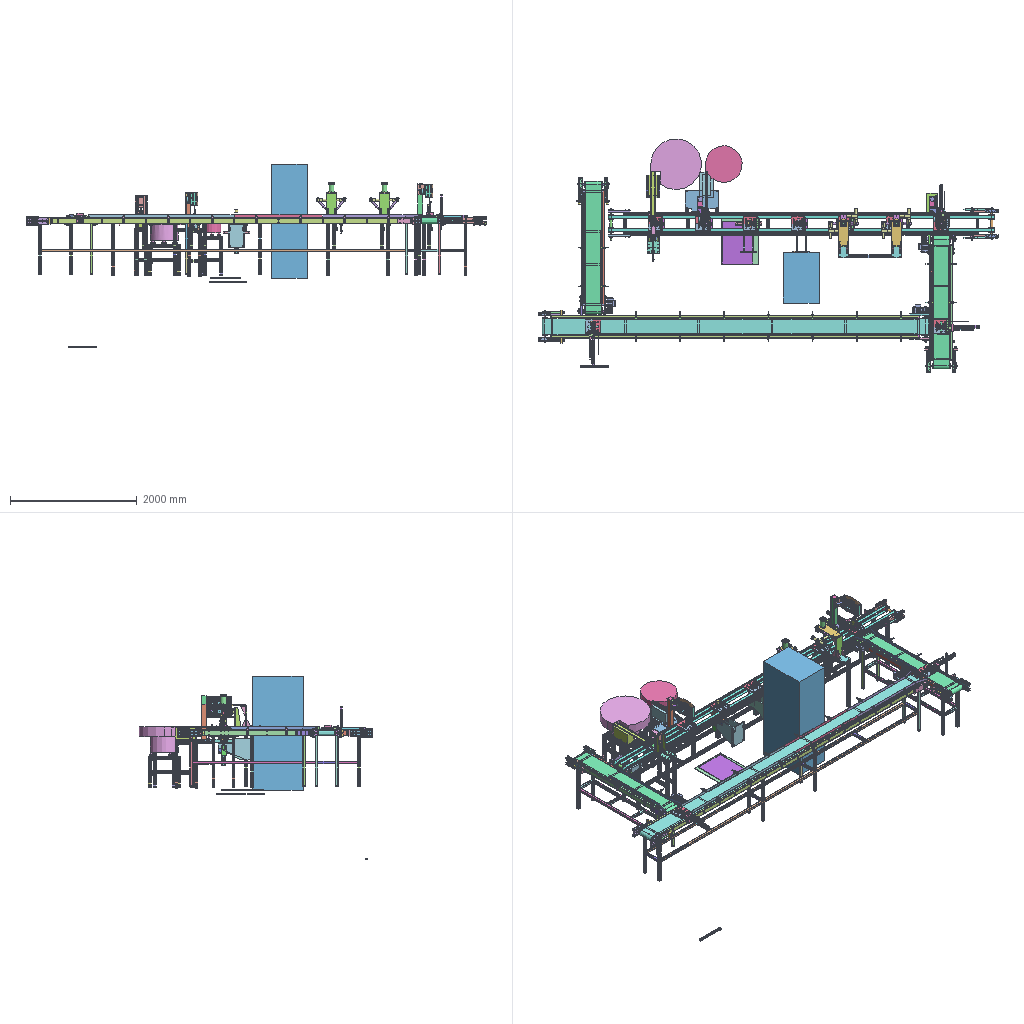Assembly | STEP file | 269 different items | 1938 placed | box 7251 x 3687 x 2899 mm
Parts list (item | name | quantity | parent item | size | volume):
1 | SN10_001_001_PLACA | x2 | in SN10_001_000_ESTEIRA | 400 x 25 x 100 mm | 770318 mm3
2 | SN10_001_002_SUPORTE | x4 | in SN10_001_000_ESTEIRA | 200 x 40 x 15 mm | 112660 mm3
3 | SN10_001_003_GUIA | x4 | in SN10_001_000_ESTEIRA | 200 x 11.9 x 27 mm | 60502 mm3
4 | SN10_001_004_PLACA | x2 | in SN10_001_000_ESTEIRA | 20 x 80 x 100 mm | 152757 mm3
5 | SN10_001_005_FUSO | x2 | in SN10_001_000_ESTEIRA | 402 x 20 x 20 mm | 117949 mm3
6 | SN10_001_006_EIXO | x1 | in SN10_001_000_ESTEIRA | 40 x 500.1 x 40 mm | 341783 mm3
7 | SN10_001_007_PLACA | x1 | in SN10_001_000_ESTEIRA | 345 x 25 x 90 mm | 704137 mm3
8 | SN10_001_008_EIXO | x1 | in SN10_001_000_ESTEIRA | 40 x 503.3 x 40 mm | 336623 mm3
9 | SN10_001_009_POLIA | x4 | in SN10_001_000_ESTEIRA | 92 x 80 x 92 mm | 413118 mm3
10 | SN10_001_010_PLACA | x1 | in SN10_001_000_ESTEIRA | 345 x 25 x 90 mm | 675174 mm3
11 | 1 | x2 | in SN10_001_011_ESTRUTURA | 5600 x 90 x 45 mm | 9330158 mm3
12 | 1_1 | x2 | in SN10_001_011_ESTRUTURA | 5510 x 45 x 45 mm | 4505764 mm3
13 | 1_2 | x4 | in SN10_001_011_ESTRUTURA | 855 x 45 x 45 mm | 699170 mm3
14 | 1_3 | x4 | in SN10_001_011_ESTRUTURA | 810 x 45 x 45 mm | 662372 mm3
15 | 1_4 | x2 | in SN10_001_011_ESTRUTURA | 680 x 45 x 45 mm | 556065 mm3
16 | 1_5 | x12 | in SN10_001_011_ESTRUTURA | 400 x 45 x 45 mm | 327097 mm3
17 | 1_6 | x4 | in SN10_001_011_ESTRUTURA | 300 x 45 x 45 mm | 245323 mm3
18 | 1_7 | x6 | in SN10_001_011_ESTRUTURA | 270 x 45 x 45 mm | 220791 mm3
19 | 1_8 | x4 | in SN10_001_011_ESTRUTURA | 245 x 45 x 45 mm | 200347 mm3
20 | 1_9 | x1 | in SN10_001_011_ESTRUTURA | 185 x 45 x 45 mm | 151282 mm3
21 | 1_10 | x1 | in SN10_001_011_ESTRUTURA | 520 x 45 x 45 mm | 425226 mm3
22 | 1_11 | x4 | in SN10_001_011_ESTRUTURA | 315 x 45 x 45 mm | 257589 mm3
23 | 1_12 | x1 | in SN10_001_011_ESTRUTURA | 985 x 45 x 45 mm | 805477 mm3
24 | 1_13 | x4 | in SN10_001_011_ESTRUTURA | 250 x 45 x 45 mm | 204436 mm3
25 | 1_14 | x2 | in SN10_001_011_ESTRUTURA | 855 x 45 x 45 mm | 699170 mm3
26 | 1_15 | x1 | in SN10_001_011_ESTRUTURA | 170 x 45 x 45 mm | 139016 mm3
27 | SN10_001_012_TRAVA | x1 | in SN10_001_000_ESTEIRA | 11 x 30 x 30 mm | 6549 mm3
28 | TU_20_TF_2_14a | x2 | in SN10_001_000_ESTEIRA | 35.3 x 92 x 97 mm | 122603 mm3
29 | 1_16 | x68 | in SN10_001_000_ESTEIRA, SN10_002_000_ESTEIRA, SN10_013_000_SISTEMA_ELEVATORIO | 13.4 x 13.4 x 2.5 mm | 205.865 mm3
30 | HABASIT_ESTEIRA | x2 | in SN10_001_000_ESTEIRA | 6090 x 50 x 90 mm | 1227646 mm3
31 | 1_17 | x36 | in SN10_001_000_ESTEIRA, SN10_002_000_ESTEIRA | 13 x 13 x 38 mm | 2414 mm3
32 | 1_18 | x48 | in SN10_001_000_ESTEIRA, SN10_002_000_ESTEIRA | 7.92 x 8 x 32 mm | 1366 mm3
33 | 1_19 | x40 | in SN10_001_000_ESTEIRA, SN10_002_000_ESTEIRA | 10 x 10 x 26 mm | 953.385 mm3
34 | 1_20 | x12 | in SN10_001_000_ESTEIRA, SN10_002_000_ESTEIRA | 13 x 13 x 43 mm | 2658 mm3
35 | 1_21 | x16 | in SN10_001_000_ESTEIRA | 19.4 x 8.5 x 45.7 mm | 2919 mm3
36 | 1_22 | x60 | in SN10_001_000_ESTEIRA, SN10_013_000_SISTEMA_ELEVATORIO, SN10_014_000_SISTEMA_BARRAGEM | 21 x 21 x 8 mm | 1207 mm3
37 | FYJ_3_4_TF_2_14a | x4 | in SN10_001_000_ESTEIRA, SN10_002_000_ESTEIRA, SN10_003_000_ESTEIRA | 33.3 x 86 x 86 mm | 78576 mm3
38 | 1_23 | x46 | in SN10_001_000_ESTEIRA, SN10_013_000_SISTEMA_ELEVATORIO, SN10_014_000_SISTEMA_BARRAGEM | 19.4 x 8.5 x 35.7 mm | 2417 mm3
39 | 1_24 | x4 | in SN10_001_000_ESTEIRA | 16.5 x 16.5 x 3 mm | 372.946 mm3
40 | 1_25 | x12 | in SN10_001_000_ESTEIRA, SN10_002_000_ESTEIRA | 16 x 16 x 50 mm | 4802 mm3
41 | 1_26 | x18 | in SN10_001_000_ESTEIRA, SN10_015_000_SISTEMA_TRANSFERENCIA, SN10_019_000_SISTEMA_DE_ABASTECIMENTO_ARRUELA | 10.4 x 10.4 x 2 mm | 101.14 mm3
42 | 1_27 | x4 | in SN10_001_000_ESTEIRA | 10 x 11.547 x 39 mm | 1326 mm3
43 | 1_28 | x1 | in SN10_001_000_ESTEIRA | 34.641 x 30 x 16 mm | 8431 mm3
44 | SN10_002_001_PLACA | x2 | in SN10_002_000_ESTEIRA | 315 x 25 x 90 mm | 605966 mm3
45 | SN10_002_002_PLACA | x2 | in SN10_002_000_ESTEIRA | 315 x 25 x 90 mm | 576590 mm3
46 | SN10_002_003_PLACA | x4 | in SN10_002_000_ESTEIRA | 20 x 80 x 100 mm | 152757 mm3
47 | SN10_002_004_PLACA | x4 | in SN10_002_000_ESTEIRA | 360 x 25 x 100 mm | 658656 mm3
48 | SN10_002_005_FUSO | x4 | in SN10_002_000_ESTEIRA | 270 x 35 x 35 mm | 89911 mm3
49 | SN10_002_006_GUIA | x8 | in SN10_002_000_ESTEIRA | 200 x 13.5 x 27 mm | 68797 mm3
50 | SN10_002_007_SUPORTE | x8 | in SN10_002_000_ESTEIRA | 200 x 40 x 15 mm | 112375 mm3
51 | SN10_002_008-01_TUBO_RETANGULAR | x2 | in SN10_002_008_ESTRUTURA | 1820 x 40 x 80 mm | 1167783 mm3
52 | SN10_002_008-02_TUBO_RETANGULAR | x4 | in SN10_002_008_ESTRUTURA | 360 x 40 x 80 mm | 211463 mm3
53 | SN10_002_008-03_TUBO_QUADRADO | x6 | in SN10_002_008_ESTRUTURA | 40 x 40 x 800 mm | 336658 mm3
54 | SN10_002_008-04_TUBO_QUADRADO | x4 | in SN10_002_008_ESTRUTURA | 1740 x 40 x 40 mm | 732232 mm3
55 | SN10_002_008-05_TUBO_QUADRADO | x8 | in SN10_002_008_ESTRUTURA | 40 x 280 x 40 mm | 117830 mm3
56 | SN10_002_008-06_TUBO_RETANGULAR | x4 | in SN10_002_008_ESTRUTURA | 40 x 280 x 80 mm | 185030 mm3
57 | SN10_002_008-07_PLACA | x8 | in SN10_002_008_ESTRUTURA | 34 x 34 x 19 mm | 18158 mm3
58 | SN10_002_008-09_TUBO_RETANGULAR | x2 | in SN10_002_008_ESTRUTURA | 1820 x 40 x 80 mm | 1165898 mm3
59 | SN10_002_008-10_TUBO_QUADRADO | x2 | in SN10_002_008_ESTRUTURA | 40 x 40 x 800 mm | 336658 mm3
60 | SN10_002_009-01_DISCO | x4 | in SN10_002_009_POLIA | 80 x 6.3 x 80 mm | 27788 mm3
61 | SN10_002_009-02_TUBO | x2 | in SN10_002_009_POLIA | 90 x 288.6 x 90 mm | 385332 mm3
62 | SN10_002_009-03_EIXO | x2 | in SN10_002_009_POLIA | 28 x 498.3 x 28 mm | 278975 mm3
63 | SN10_002_010-01_DISCO | x4 | in SN10_002_010_POLIA | 80 x 6.3 x 80 mm | 27788 mm3
64 | SN10_002_010-02_TUBO | x2 | in SN10_002_010_POLIA | 90 x 288.6 x 90 mm | 385332 mm3
65 | SN10_002_010-03_EIXO | x2 | in SN10_002_010_POLIA | 28 x 500.1 x 28 mm | 283207 mm3
66 | SN10_002_011_PLACA | x2 | in SN10_002_000_ESTEIRA | 40 x 10 x 60 mm | 22513 mm3
67 | 1_29 | x3 | in SN10_002_000_ESTEIRA, SN10_003_000_ESTEIRA | 256 x 153.5 x 121.5 mm | 2048036 mm3
68 | TU_20_TF_2_14a---(SKF) | x6 | in SN10_002_000_ESTEIRA, SN10_003_000_ESTEIRA | 35.3 x 92 x 97 mm | 122603 mm3
69 | ESTEIRA_002 | x2 | in SN10_002_000_ESTEIRA | 675.479 x 95 x 2102 mm | 2146084 mm3
70 | 1_30 | x194 | in SN10_002_000_ESTEIRA, SN10_015_000_SISTEMA_TRANSFERENCIA, SN10_016_000_SISTEMA_DE_GUIA, SN10_017_000_SISTEMA_DE_GUIA | 16.5 x 16.5 x 3 mm | 372.946 mm3
71 | 1_31 | x44 | in SN10_002_000_ESTEIRA, SN10_015_000_SISTEMA_TRANSFERENCIA | 16 x 16 x 90 mm | 7943 mm3
72 | 1_32 | x126 | in SN10_002_000_ESTEIRA, SN10_015_000_SISTEMA_TRANSFERENCIA, SN10_016_000_SISTEMA_DE_GUIA, SN10_017_000_SISTEMA_DE_GUIA | 19.63 x 17 x 8 mm | 1521 mm3
73 | SN10_003_001_PLACA | x1 | in SN10_003_000_ESTEIRA | 315 x 25 x 90 mm | 605966 mm3
74 | SN10_003_002_PLACA | x1 | in SN10_003_000_ESTEIRA | 315 x 25 x 90 mm | 578161 mm3
75 | SN10_003_003_PLACA | x2 | in SN10_003_000_ESTEIRA | 20 x 80 x 100 mm | 152757 mm3
76 | SN10_003_004_PLACA | x2 | in SN10_003_000_ESTEIRA | 360 x 25 x 100 mm | 661169 mm3
77 | SN10_003_005_FUSO | x2 | in SN10_003_000_ESTEIRA | 270 x 35 x 35 mm | 89911 mm3
78 | SN10_003_006_GUIA | x4 | in SN10_003_000_ESTEIRA | 200 x 13.5 x 27 mm | 68797 mm3
79 | SN10_003_007_SUPORTE | x4 | in SN10_003_000_ESTEIRA | 200 x 40 x 15 mm | 112375 mm3
80 | SN10_003_008-01_TUBO_RETANGULAR | x2 | in SN10_003_008_ESTRUTURA | 5820 x 40 x 80 mm | 3744159 mm3
81 | SN10_003_008-02_TUBO_RETANGULAR | x2 | in SN10_003_008_ESTRUTURA | 360 x 40 x 80 mm | 211463 mm3
82 | SN10_003_008-03_TUBO_QUADRADO | x4 | in SN10_003_008_ESTRUTURA | 40 x 40 x 800 mm | 336658 mm3
83 | SN10_003_008-04_TUBO_QUADRADO | x2 | in SN10_003_008_ESTRUTURA | 5740 x 40 x 40 mm | 2415524 mm3
84 | SN10_003_008-05_TUBO_QUADRADO | x6 | in SN10_003_008_ESTRUTURA | 40 x 280 x 40 mm | 117830 mm3
85 | SN10_003_008-06_TUBO_RETANGULAR | x4 | in SN10_003_008_ESTRUTURA | 40 x 280 x 80 mm | 185030 mm3
86 | SN10_003_008-07_PLACA | x8 | in SN10_003_008_ESTRUTURA | 34 x 34 x 19 mm | 18158 mm3
87 | SN10_003_008-08_TUBO_QUADRADO | x4 | in SN10_003_008_ESTRUTURA | 40 x 40 x 407 mm | 171275 mm3
88 | SN10_003_008-09_TUBO_QUADRADO | x4 | in SN10_003_008_ESTRUTURA | 40 x 40 x 353 mm | 148551 mm3
89 | SN10_003_009-01_DISCO | x2 | in SN10_003_009_POLIA | 80 x 6.3 x 80 mm | 27788 mm3
90 | SN10_003_009-02_TUBO | x1 | in SN10_003_009_POLIA | 90 x 288.6 x 90 mm | 385332 mm3
91 | SN10_003_009-03_EIXO | x1 | in SN10_003_009_POLIA | 28 x 498.3 x 28 mm | 277666 mm3
92 | SN10_003_010-01_DISCO | x2 | in SN10_003_010_POLIA | 80 x 6.3 x 80 mm | 27788 mm3
93 | SN10_003_010-02_TUBO | x1 | in SN10_003_010_POLIA | 90 x 288.6 x 90 mm | 385332 mm3
94 | SN10_003_010-03_EIXO | x1 | in SN10_003_010_POLIA | 28 x 500.1 x 28 mm | 283207 mm3
95 | ESTEIRA_003 | x1 | in SN10_003_000_ESTEIRA | 1498 x 95 x 6016 mm | 6146084 mm3
96 | BERCO_001 | x10 | in PRODUTO | 83.204 x 12 x 97.117 mm | 36018 mm3
97 | BERCO_002 | x10 | in PRODUTO | 247.817 x 12 x 265.596 mm | 428406 mm3
98 | BERCO_003 | x20 | in PRODUTO | 43.278 x 12 x 113.233 mm | 26889 mm3
99 | BERCO_004 | x10 | in PRODUTO | 223.963 x 12 x 154.905 mm | 182941 mm3
100 | BERCO_004_SIMETRICO | x10 | in PRODUTO | 226.019 x 12 x 152.848 mm | 182941 mm3
101 | BERCO_005 | x10 | in PRODUTO | 83.204 x 12 x 97.117 mm | 41261 mm3
102 | PARAFUSO M6x25 - DIN_912 | x40 | in PRODUTO | 31 x 10 x 10 mm | 1061 mm3
103 | PARAFUSO M4x20 - DIN_912 | x120 | in PRODUTO | 24 x 7 x 7 mm | 373.112 mm3
104 | 1_33 | x40 | in PRODUTO | 8.083 x 7 x 3.2 mm | 106.427 mm3
105 | PRODUTO_BUCHA | x10 | in Canoinha montada | 17 x 16 x 17 mm | 2259 mm3
106 | PRODUTO_PLACA | x10 | in Canoinha montada | - | -
107 | PRODUTO_ARRUELA | x13 | in Canoinha montada, SN10_006_000_ESTAGIO_2, SN10_019_000_SISTEMA_DE_ABASTECIMENTO_ARRUELA | 50 x 4.8 x 50 mm | 2970 mm3
108 | PRODUTO_PINO | x13 | in Canoinha montada, SN10_008_000_ESTAGIO_4 | 25 x 19 x 25 mm | 3402 mm3
109 | SN10_006_001_PILOTO | x1 | in SN10_006_000_ESTAGIO_2 | 30 x 100 x 30 mm | 30633 mm3
110 | SN10_006_002_PISADOR | x1 | in SN10_006_000_ESTAGIO_2 | 45.364 x 8 x 42.272 mm | 8699 mm3
111 | SN10_006_003_GUIA | x2 | in SN10_006_000_ESTAGIO_2 | 15.346 x 59 x 10.708 mm | 3098 mm3
112 | SN10_006_004_GAVETA | x1 | in SN10_006_000_ESTAGIO_2 | 122.344 x 12.5 x 315.126 mm | 195820 mm3
113 | SN10_006_005-01_PLACA | x1 | in SN10_006_005_CONJUNTO SOLDADO | 185 x 16 x 320 mm | 727969 mm3
114 | SN10_006_005-02_PLACA | x2 | in SN10_006_005_CONJUNTO SOLDADO | 50 x 91 x 15 mm | 63679 mm3
115 | SN10_006_005-03_REFORCO | x2 | in SN10_006_005_CONJUNTO SOLDADO | 16 x 80 x 310 mm | 276279 mm3
116 | SN10_006_006_SUPORTE | x2 | in SN10_006_000_ESTAGIO_2 | 65 x 158 x 19 mm | 192576 mm3
117 | SN10_006_007_PLACA | x1 | in SN10_006_000_ESTAGIO_2 | 185 x 290 x 25.5 mm | 1268482 mm3
118 | 19211 DSNU-20-80-P-A | x1 | in SN10_006_000_ESTAGIO_2 | 36.95 x 32 x 292 mm | 57538 mm3
119 | 19210 DSNU-20-50-P-A-----(asm_0_1) | x1 | in SN10_006_000_ESTAGIO_2 | 36.95 x 32 x 232 mm | 60932 mm3
120 | SHS15C-1SS-155 | x1 | in SN10_006_000_ESTAGIO_2 | 155 x 47 x 24.001 mm | 62079 mm3
121 | 2062 FK-M8 | x1 | in SN10_006_000_ESTAGIO_2 | 17 x 19 x 49 mm | 7068 mm3
122 | 1_34 | x3 | in SN10_006_000_ESTAGIO_2 | 25 x 45 x 54 mm | 12239 mm3
123 | PROJECTION BASE 1 WASHER | x2 | in MACHINE BASE PROJECTION 1 WASHER | 205 x 160 x 169 mm | 2313406 mm3
124 | SN10_013_001_PLACA | x6 | in SN10_013_000_SISTEMA_ELEVATORIO | 19 x 170 x 140 mm | 426435 mm3
125 | SN10_013_002_PINO | x12 | in SN10_013_000_SISTEMA_ELEVATORIO | 43 x 15 x 15 mm | 6907 mm3
126 | SN10_013_003_PINO_CONICO | x12 | in SN10_013_000_SISTEMA_ELEVATORIO | 58 x 15 x 15 mm | 7980 mm3
127 | MACHINE BASE PROJECTION 1 | x1 | in MACHINE BASE PROJECTION 1 WASHER | 260 x 360 x 535 mm | 5517318 mm3
128 | UPPER ELECTRODE PROJECTION 1 | x1 | in MACHINE BASE PROJECTION 1 WASHER | 48 x 48 x 50 mm | 90478 mm3
129 | base da maquina | x1 | in MACHINE BASE PROJECTION 1 WASHER | 486.837 x 663.677 x 10 mm | 3231029 mm3
130 | floor | x1 | in MACHINE BASE PROJECTION 1 WASHER | 586.14 x 746.049 x 10 mm | 4372895 mm3
131 | COMPOUND | x1 | in MACHINE BASE PROJECTION 1 WASHER | - | -
132 | SOLID | x1 | in SN10_007_001-01_PLACA | 209.056 x 12 x 193.596 mm | 339030 mm3
133 | COMPOUND | x1 | in SN10_007_001-01_PLACA | - | -
134 | SN10_007_001-02_PLACA | x2 | in Projection lift assembly | 44.646 x 150 x 159.048 mm | 285095 mm3
135 | SN10_007_001-03_PLACA | x1 | in Projection lift assembly | 103.364 x 12 x 171.387 mm | 133438 mm3
136 | SN10_007_005_PLACA | x1 | in Projection lift assembly | 168.139 x 12 x 110.165 mm | 127729 mm3
137 | 163371 DNC-50-50-PPV-A | x2 | in Projection lift assembly, SN10_009_000_ESTAGIO_5 | 64 x 64 x 279 mm | 523185 mm3
138 | placa de celeron | x1 | in Projection lift assembly | 12 x 180 x 160 mm | 345600 mm3
139 | SUPORTE | x2 | in Projection lift assembly | 165 x 80 x 12 mm | 153227 mm3
140 | SHIM SUPPORT | x2 | in Projection lift assembly | 130 x 32.9 x 50 mm | 166423 mm3
141 | COMPOUND | x1 | - | - | -
142 | SN10_008_001_PLACA | x1 | in SN10_008_000_ESTAGIO_4 | 520 x 340 x 15 mm | 2444343 mm3
143 | SN10_008_002_SUPORTE | x1 | in SN10_008_000_ESTAGIO_4 | 38 x 65 x 110 mm | 83544 mm3
144 | SN10_008_003_SUPORTE | x1 | in SN10_008_000_ESTAGIO_4 | 20 x 90 x 165.5 mm | 85051 mm3
145 | SN10_008_004_SUPORTE | x1 | in SN10_008_000_ESTAGIO_4 | 33 x 30 x 90 mm | 36222 mm3
146 | SN10_008_006-01_TUBO_QUADRADO | x1 | in SN10_008_006_CONJUNTO_SOLDADO | 80 x 80 x 546 mm | 491849 mm3
147 | SN10_008_006-02_PLACA | x2 | in SN10_008_006_CONJUNTO_SOLDADO, Copy (1) of SN10_008_006_CONJUNTO_SOLDADO | 80 x 240 x 15 mm | 283759 mm3
148 | SN10_008_006-03_PLACA | x2 | in SN10_008_006_CONJUNTO_SOLDADO, Copy (1) of SN10_008_006_CONJUNTO_SOLDADO | 80 x 15 x 160 mm | 188410 mm3
149 | SN10_008_006-04_TAMPA | x2 | in SN10_008_006_CONJUNTO_SOLDADO, Copy (1) of SN10_008_006_CONJUNTO_SOLDADO | 80 x 80 x 3 mm | 19107 mm3
150 | SN10_008_007-01_PLACA | x2 | in SN10_008_007_CONJUNTO_SOLDADO, Copy (1) of SN10_008_007_CONJUNTO_SOLDADO | 15 x 80 x 160 mm | 188607 mm3
151 | SN10_008_007-02_PLACA | x1 | in SN10_008_007_CONJUNTO_SOLDADO | 75 x 15 x 160 mm | 174675 mm3
152 | SN10_008_007-03_REFORCO | x1 | in SN10_008_007_CONJUNTO_SOLDADO | 65 x 80 x 16 mm | 55325 mm3
153 | 189171_ESG_10_SN_HA_QS_2_14b | x1 | in SN10_008_000_ESTAGIO_4 | 14 x 34.4 x 16.166 mm | 3340 mm3
154 | - | x12 | in P533616_HSP_25_AP_SD | 8.5 x 25 x 8.5 mm | 625.305 mm3
155 | - | x4 | in P533616_HSP_25_AP_SD | 82.749 x 20 x 200 mm | 243031 mm3
156 | - | x2 | in P533616_HSP_25_AP_SD | 360 x 200 x 36.871 mm | 145158 mm3
157 | - | x12 | in P533616_HSP_25_AP_SD | 8.5 x 17 x 8.5 mm | 468.225 mm3
158 | - | x2 | in P533616_HSP_25_AP_SD | 50 x 60 x 12.5 mm | 28207 mm3
159 | - | x4 | in P533616_HSP_25_AP_SD | 75.3 x 12 x 12 mm | 6099 mm3
160 | - | x4 | in P533616_HSP_25_AP_SD | 15 x 17.321 x 25 mm | 2729 mm3
161 | Senkschraube_DIN_965_M3x4 | x4 | in P533616_HSP_25_AP_SD | 5.6 x 4 x 5.6 mm | 33.649 mm3
162 | - | x4 | in P533616_HSP_25_AP_SD | 9 x 6.5 x 50 mm | 1500 mm3
163 | - | x2 | in P533616_HSP_25_AP_SD | 24 x 47 x 45 mm | 16099 mm3
164 | - | x4 | in P533616_HSP_25_AP_SD | 13 x 13 x 26.5 mm | 1380 mm3
165 | - | x22 | in P533616_HSP_25_AP_SD | 8.5 x 21 x 8.5 mm | 546.765 mm3
166 | - | x2 | in P533616_HSP_25_AP_SD | 18 x 143 x 110 mm | 148333 mm3
167 | - | x2 | in P533616_HSP_25_AP_SD | 24 x 47 x 45 mm | 16099 mm3
168 | - | x2 | in P533616_HSP_25_AP_SD | 110 x 143 x 18 mm | 148402 mm3
169 | - | x2 | in P533616_HSP_25_AP_SD | 19 x 19 x 50 mm | 7855 mm3
170 | - | x22 | in P533616_HSP_25_AP_SD | 7 x 14 x 7 mm | 255.725 mm3
171 | - | x4 | in P533616_HSP_25_AP_SD | 26.5 x 13 x 13 mm | 1379 mm3
172 | - | x6 | in P533616_HSP_25_AP_SD | 13 x 4 x 15.011 mm | 436.424 mm3
173 | Scheibe_DIN_125_1_B_8_4 | x2 | in P533616_HSP_25_AP_SD | 16 x 1.6 x 16 mm | 224.209 mm3
174 | - | x2 | in P533616_HSP_25_AP_SD | 93 x 54 x 12 mm | 19290 mm3
175 | - | x2 | in P533616_HSP_25_AP_SD | 49 x 24 x 49 mm | 37752 mm3
176 | - | x2 | in P533616_HSP_25_AP_SD | 23.2 x 10 x 250 mm | 48053 mm3
177 | - | x2 | in P533616_HSP_25_AP_SD | 15.5 x 26 x 250 mm | 83813 mm3
178 | - | x2 | in P533616_HSP_25_AP_SD | 30 x 123.5 x 10 mm | 18320 mm3
179 | - | x2 | in P533616_HSP_25_AP_SD | 28 x 28 x 35.5 mm | 17370 mm3
180 | - | x8 | in P533616_HSP_25_AP_SD | 8.5 x 30 x 8.5 mm | 723.48 mm3
181 | - | x2 | in P533616_HSP_25_AP_SD | 105.5 x 83.2 x 83.2 mm | 387227 mm3
182 | - | x2 | in P533616_HSP_25_AP_SD | 20 x 200 x 340 mm | 654587 mm3
183 | - | x2 | in P533616_HSP_25_AP_SD | 250 x 10 x 23.2 mm | 48160 mm3
184 | 5_ESTAGIO_001 | x1 | in SN10_009_000_ESTAGIO_5 | 82.899 x 120 x 82.899 mm | 294480 mm3
185 | 5_ESTAGIO_002 | x1 | in SN10_009_000_ESTAGIO_5 | 20 x 40 x 20 mm | 12566 mm3
186 | 5_ESTAGIO_003-01 | x1 | in 5_ESTAGIO_003 | 209.056 x 20 x 193.596 mm | 576000 mm3
187 | 5_ESTAGIO_003-02 | x2 | in 5_ESTAGIO_003 | 48.561 x 150 x 159.871 mm | 384000 mm3
188 | 5_ESTAGIO_003-03 | x1 | in 5_ESTAGIO_003 | 119.022 x 16 x 174.677 mm | 225280 mm3
189 | 5_ESTAGIO_004-01 | x2 | in 5_ESTAGIO_004 | 125.479 x 285 x 508.106 mm | 2421288 mm3
190 | 5_ESTAGIO_004-02 | x1 | in 5_ESTAGIO_004 | 263.449 x 360 x 74.068 mm | 1908000 mm3
191 | 5_ESTAGIO_005 | x1 | in SN10_009_000_ESTAGIO_5 | 173.032 x 16 x 111.193 mm | 184694 mm3
192 | SHS15C12030_Track | x4 | in SHS15C1SS120300PB1021B27.8000 | 120 x 13 x 15 mm | 19221 mm3
193 | SHS15CSSPB1021B_Slide25_55 | x4 | in SHS15C1SS120300PB1021B27.8000 | 64.4 x 21 x 47 mm | 41845 mm3
194 | 5_ESTAGIO_MAQUINA | x1 | in SN10_009_000_ESTAGIO_5 | 717.439 x 1800 x 899.09 mm | 813600000 mm3
195 | SN10_010_001_SUPORTE | x8 | in SN10_010_000_ESTAGIO_6, SN10_011_000_ESTAGIO_7 | 40 x 260 x 50 mm | 323681 mm3
196 | SN10_010_002_SUPORTE | x2 | in SN10_010_000_ESTAGIO_6, SN10_011_000_ESTAGIO_7 | 100 x 300 x 19 mm | 495492 mm3
197 | SN10_010_003_SUPORTE | x4 | in SN10_010_000_ESTAGIO_6, SN10_011_000_ESTAGIO_7 | 40 x 50 x 75 mm | 100062 mm3
198 | SN10_010_004_EIXO | x2 | in SN10_010_000_ESTAGIO_6, SN10_011_000_ESTAGIO_7 | 60 x 60 x 50 mm | 51834 mm3
199 | SN10_010_005-01_PLACA | x2 | in SN10_010_005_CONJUNTO_SOLDADO | 150 x 80 x 19 mm | 223453 mm3
200 | SN10_010_005-02_PLACA | x2 | in SN10_010_005_CONJUNTO_SOLDADO | 150 x 19 x 362.5 mm | 1033125 mm3
201 | SN10_010_005-03_REFORCO | x12 | in SN10_010_005_CONJUNTO_SOLDADO | 19 x 70 x 137 mm | 117421 mm3
202 | SN10_010_005-04_PLACA | x2 | in SN10_010_005_CONJUNTO_SOLDADO | 150 x 360 x 20 mm | 1065035 mm3
203 | SN10_010_006_PLACA | x2 | in SN10_010_000_ESTAGIO_6, SN10_011_000_ESTAGIO_7 | 150 x 425 x 19 mm | 1079785 mm3
204 | TOCHA_DE_SOLDA_TBI | x4 | in SN10_010_000_ESTAGIO_6, SN10_011_000_ESTAGIO_7 | 38 x 348 x 38 mm | 253151 mm3
205 | COMPOUND | x2 | in PE0902 | - | -
206 | SOLID | x2 | in PE0902 | 192.5 x 90 x 90 mm | 903685 mm3
207 | COMPOUND | x2 | in P0405300101 | - | -
208 | SOLID | x2 | in P0405300101 | 92 x 92 x 23.5 mm | 95291 mm3
209 | PARAFUSO_DIN 912_M8x30 | x2 | in SN10_010_000_ESTAGIO_6, SN10_011_000_ESTAGIO_7 | 38 x 13 x 13 mm | 2340 mm3
210 | 1254052_DHPS_35_A_2_14a---(CORPO) | x1 | in 1254052_DHPS_35_A_2_14a---(FESTO) | 45 x 110 x 88 mm | 385096 mm3
211 | 1254052_DHPS_35_A_2_14a---(GARRA) | x2 | in 1254052_DHPS_35_A_2_14a---(FESTO) | 20 x 55.5 x 42.5 mm | 31534 mm3
212 | SN10_012_001_GARRA | x2 | in SN10_012_000_ESTAGIO_8 | 19 x 39 x 63 mm | 23093 mm3
213 | 540883_HAPG_72_B_2_14b | x1 | in SN10_012_000_ESTAGIO_8 | 47 x 60 x 63.5 mm | 42972 mm3
214 | SN10_012_002_ADAPTADOR | x1 | in SN10_012_000_ESTAGIO_8 | 50 x 90 x 15 mm | 62180 mm3
215 | ISO 4762 SCREW M8x20 STEEL HEXAGON SOCKET HEAD CAP | x2 | in SN10_012_000_ESTAGIO_8 | 28 x 13 x 13 mm | 1862 mm3
216 | Copy (1) of SN10_008_006-01_TUBO_QUADRADO | x1 | in Copy (1) of SN10_008_006_CONJUNTO_SOLDADO | 80 x 80 x 507.179 mm | 456879 mm3
217 | Copy (1) of SN10_008_007-02_PLACA | x1 | in Copy (1) of SN10_008_007_CONJUNTO_SOLDADO | 120 x 15 x 160 mm | 282675 mm3
218 | Copy (1) of SN10_008_007-03_REFORCO | x1 | in Copy (1) of SN10_008_007_CONJUNTO_SOLDADO | 110 x 80 x 16 mm | 89525 mm3
219 | SN10_012_002_PLACA | x1 | in SN10_012_000_ESTAGIO_8 | 170 x 295 x 15 mm | 749791 mm3
220 | 189654 HMBN-5-M5-189654 HMBN-5-M5 | x2 | in SN10_012_000_ESTAGIO_8 | 7.6 x 5.445 x 12 mm | 233.461 mm3
221 | SN10_013_004_PLACA | x5 | in SN10_013_000_SISTEMA_ELEVATORIO | 10 x 360 x 100 mm | 258052 mm3
222 | - | x5 | in 170858 DFM-32-50-P-A-GF---(FESTO) | 98 x 49 x 110 mm | 384442 mm3
223 | - | x5 | in 170858 DFM-32-50-P-A-GF---(FESTO) | 131 x 47 x 108 mm | 163478 mm3
224 | 1_35 | x20 | in SN10_013_000_SISTEMA_ELEVATORIO | 8.5 x 8.5 x 35 mm | 827.103 mm3
225 | 1_36 | x20 | in SN10_013_000_SISTEMA_ELEVATORIO | 13 x 13 x 33 mm | 2162 mm3
226 | 1_37 | x24 | in SN10_013_000_SISTEMA_ELEVATORIO, SN10_019_000_SISTEMA_DE_ABASTECIMENTO_ARRUELA | 8.3 x 8.3 x 1.5 mm | 44.494 mm3
227 | SN10_014_001_PINO | x6 | in SN10_014_000_SISTEMA_BARRAGEM | 20 x 20 x 40 mm | 11102 mm3
228 | SN10_014_002-01_PLACA | x6 | in SN10_014_002_CONJUNTO_SOLDADO | 50 x 360 x 12.5 mm | 206301 mm3
229 | SN10_014_002-02_TUBO | x6 | in SN10_014_002_CONJUNTO_SOLDADO | 50 x 50 x 80 mm | 129371 mm3
230 | - | x6 | in 19210 DSNU-20-50-P-A-----(FESTO) | 27 x 27 x 158 mm | 40169 mm3
231 | - | x6 | in 19210 DSNU-20-50-P-A-----(FESTO) | 20 x 20 x 142 mm | 8430 mm3
232 | SN10_015_001_CHAPA_DOBRADA | x3 | in SN10_015_000_SISTEMA_TRANSFERENCIA | 485 x 210 x 19 mm | 177968 mm3
233 | SN10_015_002_PLACA | x3 | in SN10_015_000_SISTEMA_TRANSFERENCIA | 25 x 110 x 160 mm | 292195 mm3
234 | SN10_015_003_GUIA | x3 | in SN10_015_000_SISTEMA_TRANSFERENCIA | 380 x 10 x 10 mm | 29333 mm3
235 | SN10_015_004_BUCHA | x3 | in SN10_015_000_SISTEMA_TRANSFERENCIA | 25 x 20 x 20 mm | 5796 mm3
236 | 163314 DNC-32-320-PPV-A---(FESTO)_CORPO | x3 | in 163314 DNC-32-320-PPV-A---(FESTO) | 45 x 45 x 436 mm | 470774 mm3
237 | 163314 DNC-32-320-PPV-A---(FESTO)_HASTE | x3 | in 163314 DNC-32-320-PPV-A---(FESTO) | 32 x 32 x 415 mm | 50245 mm3
238 | 1_38 | x12 | in SN10_015_000_SISTEMA_TRANSFERENCIA | 10 x 10 x 46 mm | 1516 mm3
239 | SN10_016_001-01_CHAPA | x4 | in SN10_016_001_GUIA | 56.488 x 1320 x 45 mm | 179098 mm3
240 | SN10_016_001-02_BLOCO | x8 | in SN10_016_001_GUIA | 20 x 20 x 45 mm | 16964 mm3
241 | SN10_016_002_SUPORTE | x22 | in SN10_016_000_SISTEMA_DE_GUIA, SN10_017_000_SISTEMA_DE_GUIA | 3 x 30 x 135 mm | 11295 mm3
242 | SN10_016_003_EIXO | x22 | in SN10_016_000_SISTEMA_DE_GUIA, SN10_017_000_SISTEMA_DE_GUIA | 120 x 10 x 10 mm | 9417 mm3
243 | 1_39 | x16 | in SN10_016_000_SISTEMA_DE_GUIA | 16 x 16 x 80 mm | 7147 mm3
244 | SN10_017_001-01_CHAPA | x2 | in SN10_017_001_GUIA | 1494 x 56.488 x 45 mm | 202588 mm3
245 | SN10_017_001-02_BLOCO | x14 | in SN10_017_001_GUIA, SN10_017_002_GUIA, SN10_017_003_GUIA | 20 x 20 x 45 mm | 17008 mm3
246 | SN10_017_002-01_CHAPA | x2 | in SN10_017_002_GUIA | 1382 x 3 x 45 mm | 186570 mm3
247 | SN10_017_003-01_CHAPA | x2 | in SN10_017_003_GUIA | 2283 x 3 x 45 mm | 308205 mm3
248 | bosch_3842990520_4ea8orsd7ktxgd8l9ys4v93ta | x4 | in SN10_019_001_ALUMINUM_STRUCTURE | 485 x 45 x 45 mm | 396605 mm3
249 | bosch_3842990520_4g1k76bwvav0hbf1r78r1itfr | x11 | in SN10_019_001_ALUMINUM_STRUCTURE | 410 x 45 x 45 mm | 335275 mm3
250 | bosch_3842529383_ce331vk4hpgd1h6tci1llkgc1 | x20 | in SN10_019_001_ALUMINUM_STRUCTURE | 38 x 47.7 x 47.7 mm | 18640 mm3
251 | bosch_3842990520_1jcimurca0n3y5im9bxpmvpzt | x8 | in SN10_019_002_ALUMINUM_STRUCTURE, SN10_020_002_ALUMINUM_STRUCTURE | 740 x 45 x 45 mm | 605130 mm3
252 | bosch_3842990520_2f8lx2d0pfreq4lhyqg120tj6 | x12 | in SN10_019_002_ALUMINUM_STRUCTURE, SN10_020_002_ALUMINUM_STRUCTURE | 270 x 45 x 45 mm | 220791 mm3
253 | bosch_3842990520_bbw6j7b49i4caf90m9u0fayle | x8 | in SN10_019_002_ALUMINUM_STRUCTURE, SN10_020_002_ALUMINUM_STRUCTURE | 122 x 45 x 45 mm | 99765 mm3
254 | SN10_019_003_SUPORTE | x1 | in SN10_019_000_SISTEMA_DE_ABASTECIMENTO_ARRUELA | 16 x 161 x 147.15 mm | 54772 mm3
255 | 2_ESTAGIO_006-01 | x1 | in 2_ESTAGIO_006 | 85.161 x 5 x 93.664 mm | 26952 mm3
256 | 2_ESTAGIO_006-02 | x1 | in 2_ESTAGIO_006 | 25.4 x 30 x 25.4 mm | 10290 mm3
257 | 2_ESTAGIO_010 | x1 | in SN10_019_000_SISTEMA_DE_ABASTECIMENTO_ARRUELA | 109.627 x 12.7 x 98.805 mm | 71258 mm3
258 | 2_ESTAGIO_005 | x1 | in SN10_019_000_SISTEMA_DE_ABASTECIMENTO_ARRUELA | 10 x 15 x 10 mm | 994.545 mm3
259 | 19183 DSNU-10-10-P-A | x1 | in SN10_019_000_SISTEMA_DE_ABASTECIMENTO_ARRUELA | 15 x 15 x 106 mm | 9040 mm3
260 | CALHA_VIBRATORIA_ARRUELA | x1 | in SN10_019_000_SISTEMA_DE_ABASTECIMENTO_ARRUELA | 700 x 132 x 200 mm | 8382102 mm3
261 | ALIMENTADOR_ARRUELA | x1 | in SN10_019_000_SISTEMA_DE_ABASTECIMENTO_ARRUELA | 800 x 800 x 450 mm | 113086598 mm3
262 | DIN_912 - M5x16 | x4 | in SN10_019_000_SISTEMA_DE_ABASTECIMENTO_ARRUELA | 21 x 8.5 x 8.5 mm | 538.828 mm3
263 | DISCO_BASE_ALIMENTADOR_ARRUELA | x3 | in SN10_019_000_SISTEMA_DE_ABASTECIMENTO_ARRUELA | 70 x 70 x 10 mm | 27729 mm3
264 | bosch_3842990520_3kqsoefwhpgbs6igd9j6s2bp3 | x4 | in SN10_020_001_ALUMINUM_STRUCTURE | 610 x 45 x 45 mm | 498823 mm3
265 | bosch_3842990520_akhtc56kol25hyvavz80csddc | x11 | in SN10_020_001_ALUMINUM_STRUCTURE | 255 x 45 x 45 mm | 208524 mm3
266 | ALIMENTADOR_PINO | x1 | in SN10_020_000_SISTEMA_DE_ABASTECIMENTO_PINO | 580 x 580 x 320 mm | 38023743 mm3
267 | CALHA_VIBRATORIA_PINO | x1 | in SN10_020_000_SISTEMA_DE_ABASTECIMENTO_PINO | 600 x 212 x 235 mm | 9636960 mm3
268 | DISCO_BASE_ALIMENTADOR_PINO | x3 | in SN10_020_000_SISTEMA_DE_ABASTECIMENTO_PINO | 52 x 52 x 10 mm | 17173 mm3
269 | PERFIL_30X30_450 | x2 | in _SN10_000_000_PROJETO_CANOINHA_KEIPER | 450 x 30 x 30 mm | 139687 mm3
Placements (level | parent | child | x y z in mm | rotation matrix by rows), first 188 of 2061 lines:
1 | Canoinha | _SN10_000_000_PROJETO_CANOINHA_KEIPER | 0.0 0.0 0.0 | 1 0 0 0 1 0 0 0 1
2 | _SN10_000_000_PROJETO_CANOINHA_KEIPER | SN10_001_000_ESTEIRA | 0.0 0.0 0.0 | 1 0 0 0 1 0 0 0 1
3 | SN10_001_000_ESTEIRA | SN10_001_001_PLACA | 6000.0 -0.0 0.0 | -1 0 0 0 -1 0 0 0 1
3 | SN10_001_000_ESTEIRA | SN10_001_001_PLACA | 6000.0 -0.0 0.0 | -1 0 0 0 1 0 0 0 -1
3 | SN10_001_000_ESTEIRA | SN10_001_002_SUPORTE | 6000.0 -0.0 0.0 | -1 0 0 0 -1 0 0 0 1
3 | SN10_001_000_ESTEIRA | SN10_001_002_SUPORTE | 6000.0 -0.0 0.0 | 1 0 0 0 -1 0 0 0 -1
3 | SN10_001_000_ESTEIRA | SN10_001_002_SUPORTE | 6000.0 -0.0 0.0 | 1 0 0 0 1 0 0 0 1
3 | SN10_001_000_ESTEIRA | SN10_001_002_SUPORTE | 6000.0 -0.0 0.0 | -1 0 0 0 1 0 0 0 -1
3 | SN10_001_000_ESTEIRA | SN10_001_003_GUIA | 6000.0 -0.0 0.0 | -1 0 0 0 -1 0 0 0 1
3 | SN10_001_000_ESTEIRA | SN10_001_003_GUIA | 6000.0 -0.0 0.0 | 1 0 0 0 -1 0 0 0 -1
3 | SN10_001_000_ESTEIRA | SN10_001_003_GUIA | 6000.0 -0.0 0.0 | 1 0 0 0 1 0 0 0 1
3 | SN10_001_000_ESTEIRA | SN10_001_003_GUIA | 6000.0 -0.0 0.0 | -1 0 0 0 1 0 0 0 -1
3 | SN10_001_000_ESTEIRA | SN10_001_004_PLACA | 6000.0 -0.0 0.0 | -1 0 0 0 -1 0 0 0 1
3 | SN10_001_000_ESTEIRA | SN10_001_004_PLACA | 6000.0 -0.0 0.0 | -1 0 0 0 1 0 0 0 -1
3 | SN10_001_000_ESTEIRA | SN10_001_005_FUSO | 6000.0 -0.0 0.0 | -1 0 0 0 -1 0 0 0 1
3 | SN10_001_000_ESTEIRA | SN10_001_005_FUSO | 6000.0 442.7 0.0 | -1 0 0 0 -1 0 0 0 1
3 | SN10_001_000_ESTEIRA | SN10_001_006_EIXO | 6000.0 -0.0 0.0 | -1 0 0 0 -1 0 0 0 1
3 | SN10_001_000_ESTEIRA | SN10_001_007_PLACA | 6000.0 -0.0 0.0 | -1 0 0 0 1 0 0 0 -1
3 | SN10_001_000_ESTEIRA | SN10_001_008_EIXO | 6000.0 -0.0 0.0 | -1 0 0 0 -1 0 0 0 1
3 | SN10_001_000_ESTEIRA | SN10_001_009_POLIA | 6000.0 -0.0 0.0 | -1 0 0 0 -1 0 0 0 1
3 | SN10_001_000_ESTEIRA | SN10_001_009_POLIA | 6000.0 -200.0 0.0 | -1 0 0 0 -1 0 0 0 1
3 | SN10_001_000_ESTEIRA | SN10_001_009_POLIA | 12000.0 -0.0 0.0 | -1 0 0 0 -1 0 0 0 1
3 | SN10_001_000_ESTEIRA | SN10_001_009_POLIA | 12000.0 -200.0 0.0 | -1 0 0 0 -1 0 0 0 1
3 | SN10_001_000_ESTEIRA | SN10_001_010_PLACA | 6000.0 -0.0 0.0 | -1 0 0 0 -1 0 0 0 1
3 | SN10_001_000_ESTEIRA | SN10_001_011_ESTRUTURA | 0.0 0.0 0.0 | 1 0 0 0 1 0 0 0 1
4 | SN10_001_011_ESTRUTURA | 1 | 200.0 157.5 0.0 | 1 0 0 0 0 1 0 -1 0
4 | SN10_001_011_ESTRUTURA | 1 | 200.0 -157.5 0.0 | 1 0 0 0 0 1 0 -1 0
4 | SN10_001_011_ESTRUTURA | 1_1 | 134.371 157.5 -467.5 | 1 0 0 0 1 0 0 0 1
4 | SN10_001_011_ESTRUTURA | 1_1 | 134.371 -157.5 -467.5 | 1 0 0 0 1 0 0 0 1
4 | SN10_001_011_ESTRUTURA | 1_2 | 4552.5 -517.5 0.0 | 0 0 -1 0 -1 0 -1 0 0
4 | SN10_001_011_ESTRUTURA | 1_2 | 736.371 -447.5 -0.0 | 0 0 -1 0 -1 0 -1 0 0
4 | SN10_001_011_ESTRUTURA | 1_3 | 222.5 157.5 -855.0 | 0 0 1 0 -1 0 1 0 0
4 | SN10_001_011_ESTRUTURA | 1_3 | 222.5 -157.5 -855.0 | 0 0 1 0 -1 0 1 0 0
4 | SN10_001_011_ESTRUTURA | 1_3 | 5777.5 157.5 -855.0 | 0 0 1 0 -1 0 1 0 0
4 | SN10_001_011_ESTRUTURA | 1_3 | 5777.5 -157.5 -855.0 | 0 0 1 0 -1 0 1 0 0
4 | SN10_001_011_ESTRUTURA | 1_4 | 1195.588 502.5 -175 | 0 0 1 0 1 0 -1 0 0
4 | SN10_001_011_ESTRUTURA | 1_4 | 1670.588 502.5 -175 | 0 0 1 0 1 0 -1 0 0
4 | SN10_001_011_ESTRUTURA | 1_5 | 707.0 157.5 -445.0 | 0 0 1 0 -1 0 1 0 0
4 | SN10_001_011_ESTRUTURA | 1_5 | 1195.588 157.5 -445.0 | 0 0 1 0 -1 0 1 0 0
4 | SN10_001_011_ESTRUTURA | 1_5 | 3707.0 157.5 -445.0 | 0 0 1 0 -1 0 1 0 0
4 | SN10_001_011_ESTRUTURA | 1_5 | 4457.0 157.5 -445.0 | 0 0 1 0 -1 0 1 0 0
4 | SN10_001_011_ESTRUTURA | 1_5 | 707.0 -157.5 -445.0 | 0 0 1 0 -1 0 1 0 0
4 | SN10_001_011_ESTRUTURA | 1_5 | 1457.0 -157.5 -445.0 | 0 0 1 0 -1 0 1 0 0
4 | SN10_001_011_ESTRUTURA | 1_5 | 3707.0 -157.5 -445.0 | 0 0 1 0 -1 0 1 0 0
4 | SN10_001_011_ESTRUTURA | 1_5 | 4457.0 -157.5 -445.0 | 0 0 1 0 -1 0 1 0 0
4 | SN10_001_011_ESTRUTURA | 1_6 | 1670.588 180.0 -467.5 | 0 0 -1 1 0 0 0 -1 0
4 | SN10_001_011_ESTRUTURA | 1_6 | 1195.588 180.0 -467.5 | 0 0 -1 1 0 0 0 -1 0
4 | SN10_001_011_ESTRUTURA | 1_6 | 1195.588 180.0 -152.5 | 0 0 -1 1 0 0 0 -1 0
4 | SN10_001_011_ESTRUTURA | 1_6 | 1670.588 180.0 -152.5 | 0 0 -1 1 0 0 0 -1 0
4 | SN10_001_011_ESTRUTURA | 1_7 | 222.5 135.0 -467.5 | 0 1 0 -1 0 0 0 0 1
4 | SN10_001_011_ESTRUTURA | 1_7 | 5777.5 135.0 -467.5 | 0 1 0 -1 0 0 0 0 1
4 | SN10_001_011_ESTRUTURA | 1_8 | 736.371 -425.0 22.5 | 0 1 0 1 0 0 0 0 -1
4 | SN10_001_011_ESTRUTURA | 1_8 | 596.371 -425.0 22.5 | 0 1 0 1 0 0 0 0 -1
4 | SN10_001_011_ESTRUTURA | 1_8 | 596.371 -425.0 -467.5 | 0 1 0 1 0 0 0 0 -1
4 | SN10_001_011_ESTRUTURA | 1_8 | 736.371 -425.0 -467.5 | 0 1 0 1 0 0 0 0 -1
4 | SN10_001_011_ESTRUTURA | 1_9 | 573.871 -447.5 22.5 | 1 0 0 0 1 0 0 0 1
4 | SN10_001_011_ESTRUTURA | 1_5 | 1670.588 157.5 -445.0 | 0 0 1 0 -1 0 1 0 0
4 | SN10_001_011_ESTRUTURA | 1_5 | 1457.0 157.5 -445.0 | 0 0 1 0 -1 0 1 0 0
4 | SN10_001_011_ESTRUTURA | 1_10 | 1173.088 502.5 -152.5 | 1 0 0 0 1 0 0 0 1
4 | SN10_001_011_ESTRUTURA | 1_5 | 5207.0 157.5 -445.0 | 0 0 1 0 -1 0 1 0 0
4 | SN10_001_011_ESTRUTURA | 1_5 | 5207.0 -157.5 -445.0 | 0 0 1 0 -1 0 1 0 0
4 | SN10_001_011_ESTRUTURA | 1_7 | 4677.5 135.0 -467.5 | 0 1 0 -1 0 0 0 0 1
4 | SN10_001_011_ESTRUTURA | 1_7 | 3577.5 135.0 -467.5 | 0 1 0 -1 0 0 0 0 1
4 | SN10_001_011_ESTRUTURA | 1_7 | 2477.5 135.0 -467.5 | 0 1 0 -1 0 0 0 0 1
4 | SN10_001_011_ESTRUTURA | 1_7 | 1212.162 135.0 -467.5 | 0 1 0 -1 0 0 0 0 1
4 | SN10_001_011_ESTRUTURA | 1_11 | 3717.5 -580.0 22.5 | 0 0 1 1 0 0 0 1 0
4 | SN10_001_011_ESTRUTURA | 1_11 | 4552.5 -580.0 22.5 | 0 0 1 1 0 0 0 1 0
4 | SN10_001_011_ESTRUTURA | 1_11 | 4447.5 -580.0 22.5 | 0 0 1 1 0 0 0 1 0
4 | SN10_001_011_ESTRUTURA | 1_11 | 3612.5 -580.0 22.5 | 0 0 1 1 0 0 0 1 0
4 | SN10_001_011_ESTRUTURA | 1_12 | 3990.0 -517.5 22.5 | -1 0 0 0 0 1 0 1 0
4 | SN10_001_011_ESTRUTURA | 1_2 | 3612.5 -517.5 0.0 | 0 0 -1 0 -1 0 -1 0 0
4 | SN10_001_011_ESTRUTURA | 1_2 | 596.371 -447.5 -0.0 | 0 0 -1 0 -1 0 -1 0 0
4 | SN10_001_011_ESTRUTURA | 1_13 | 4999.0 580.0 -467.5 | 0 0 1 -1 0 0 0 -1 0
4 | SN10_001_011_ESTRUTURA | 1_13 | 5124.0 580.0 -469.5 | 0 0 1 -1 0 0 0 -1 0
4 | SN10_001_011_ESTRUTURA | 1_14 | 4999.0 452.5 -355.0 | 0 0 1 0 -1 0 1 0 0
4 | SN10_001_011_ESTRUTURA | 1_14 | 5124.0 452.5 -355.0 | 0 0 1 0 -1 0 1 0 0
4 | SN10_001_011_ESTRUTURA | 1_13 | 4999.0 580.0 22.5 | 0 0 1 -1 0 0 0 -1 0
4 | SN10_001_011_ESTRUTURA | 1_13 | 5124.0 580.0 22.5 | 0 0 1 -1 0 0 0 -1 0
4 | SN10_001_011_ESTRUTURA | 1_15 | 5296.5 452.5 22.5 | -1 0 0 0 0 -1 0 -1 0
3 | SN10_001_000_ESTEIRA | SN10_001_012_TRAVA | 0.0 0.0 0.0 | 1 0 0 0 1 0 0 0 1
3 | SN10_001_000_ESTEIRA | TU_20_TF_2_14a | 6000.0 -221.75 0.0 | 0 0 1 -1 0 0 0 -1 0
3 | SN10_001_000_ESTEIRA | TU_20_TF_2_14a | 6000.0 220.95 0.0 | 0 0 1 1 0 0 0 1 0
3 | SN10_001_000_ESTEIRA | 1_16 | 5915.0 -187.5 65.0 | -1 0 0 0 -1 0 0 0 1
3 | SN10_001_000_ESTEIRA | HABASIT_ESTEIRA | 0.0 0.0 0.0 | 1 0 0 0 1 0 0 0 1
3 | SN10_001_000_ESTEIRA | HABASIT_ESTEIRA | 0.0 -200.0 -0.0 | 1 0 0 0 1 0 0 0 1
3 | SN10_001_000_ESTEIRA | 1_16 | 6000.0 -187.5 65.0 | -1 0 0 0 -1 0 0 0 1
3 | SN10_001_000_ESTEIRA | 1_16 | 6085.0 -187.5 65.0 | -1 0 0 0 -1 0 0 0 1
3 | SN10_001_000_ESTEIRA | 1_16 | 5915.0 187.5 65.0 | -1 0 0 0 -1 0 0 0 1
3 | SN10_001_000_ESTEIRA | 1_16 | 6000.0 187.5 65.0 | -1 0 0 0 -1 0 0 0 1
3 | SN10_001_000_ESTEIRA | 1_16 | 6085.0 187.5 65.0 | -1 0 0 0 -1 0 0 0 1
3 | SN10_001_000_ESTEIRA | 1_16 | 5915.0 -187.5 -67.5 | -1 0 0 0 -1 0 0 0 1
3 | SN10_001_000_ESTEIRA | 1_16 | 6000.0 -187.5 -67.5 | -1 0 0 0 -1 0 0 0 1
3 | SN10_001_000_ESTEIRA | 1_16 | 6085.0 -187.5 -67.5 | -1 0 0 0 -1 0 0 0 1
3 | SN10_001_000_ESTEIRA | 1_16 | 5915.0 187.5 -67.5 | -1 0 0 0 -1 0 0 0 1
3 | SN10_001_000_ESTEIRA | 1_16 | 6000.0 187.5 -67.5 | -1 0 0 0 -1 0 0 0 1
3 | SN10_001_000_ESTEIRA | 1_16 | 6085.0 187.5 -67.5 | -1 0 0 0 -1 0 0 0 1
3 | SN10_001_000_ESTEIRA | 1_17 | 5915.0 -187.5 67.5 | -1 0 0 0 -1 0 0 0 1
3 | SN10_001_000_ESTEIRA | 1_17 | 6000.0 -187.5 67.5 | -1 0 0 0 -1 0 0 0 1
3 | SN10_001_000_ESTEIRA | 1_17 | 6085.0 -187.5 67.5 | -1 0 0 0 -1 0 0 0 1
3 | SN10_001_000_ESTEIRA | 1_17 | 5915.0 187.5 67.5 | -1 0 0 0 -1 0 0 0 1
3 | SN10_001_000_ESTEIRA | 1_17 | 6000.0 187.5 67.5 | -1 0 0 0 -1 0 0 0 1
3 | SN10_001_000_ESTEIRA | 1_17 | 6085.0 187.5 67.5 | -1 0 0 0 -1 0 0 0 1
3 | SN10_001_000_ESTEIRA | 1_17 | 5915.0 -187.5 -67.5 | 1 0 0 0 -1 0 0 0 -1
3 | SN10_001_000_ESTEIRA | 1_17 | 6000.0 -187.5 -67.5 | 1 0 0 0 -1 0 0 0 -1
3 | SN10_001_000_ESTEIRA | 1_17 | 6085.0 -187.5 -67.5 | 1 0 0 0 -1 0 0 0 -1
3 | SN10_001_000_ESTEIRA | 1_17 | 5915.0 187.5 -67.5 | 1 0 0 0 -1 0 0 0 -1
3 | SN10_001_000_ESTEIRA | 1_17 | 6000.0 187.5 -67.5 | 1 0 0 0 -1 0 0 0 -1
3 | SN10_001_000_ESTEIRA | 1_17 | 6085.0 187.5 -67.5 | 1 0 0 0 -1 0 0 0 -1
3 | SN10_001_000_ESTEIRA | 1_18 | 5957.5 187.5 65.0 | 1 0 0 0 -1 0 0 0 -1
3 | SN10_001_000_ESTEIRA | 1_18 | 6042.5 187.5 65.0 | 1 0 0 0 -1 0 0 0 -1
3 | SN10_001_000_ESTEIRA | 1_18 | 5957.5 -187.5 65.0 | 1 0 0 0 -1 0 0 0 -1
3 | SN10_001_000_ESTEIRA | 1_18 | 6042.5 -187.5 65.0 | 1 0 0 0 -1 0 0 0 -1
3 | SN10_001_000_ESTEIRA | 1_18 | 5957.5 -187.5 -65.0 | -1 0 0 0 -1 0 0 0 1
3 | SN10_001_000_ESTEIRA | 1_18 | 6042.5 -187.5 -65.0 | -1 0 0 0 -1 0 0 0 1
3 | SN10_001_000_ESTEIRA | 1_18 | 5957.5 187.5 -65.0 | -1 0 0 0 -1 0 0 0 1
3 | SN10_001_000_ESTEIRA | 1_18 | 6042.5 187.5 -65.0 | -1 0 0 0 -1 0 0 0 1
3 | SN10_001_000_ESTEIRA | 1_18 | 5915.0 -228.5 57.5 | 1 0 0 0 0 1 0 -1 0
3 | SN10_001_000_ESTEIRA | 1_18 | 6085.0 -228.5 57.5 | 1 0 0 0 0 1 0 -1 0
3 | SN10_001_000_ESTEIRA | 1_18 | 5915.0 -228.5 -57.5 | 1 0 0 0 0 1 0 -1 0
3 | SN10_001_000_ESTEIRA | 1_18 | 6085.0 -228.5 -57.5 | 1 0 0 0 0 1 0 -1 0
3 | SN10_001_000_ESTEIRA | 1_18 | 5915.0 228.5 57.5 | 1 0 0 0 0 -1 0 1 0
3 | SN10_001_000_ESTEIRA | 1_18 | 6085.0 228.5 57.5 | 1 0 0 0 0 -1 0 1 0
3 | SN10_001_000_ESTEIRA | 1_18 | 5915.0 228.5 -57.5 | 1 0 0 0 0 -1 0 1 0
3 | SN10_001_000_ESTEIRA | 1_18 | 6085.0 228.5 -57.5 | 1 0 0 0 0 -1 0 1 0
3 | SN10_001_000_ESTEIRA | 1_19 | 5940.0 -221.5 57.5 | -1 0 0 0 0 -1 0 -1 0
3 | SN10_001_000_ESTEIRA | 1_19 | 6000.0 -221.5 57.5 | -1 0 0 0 0 -1 0 -1 0
3 | SN10_001_000_ESTEIRA | 1_19 | 6060.0 -221.5 57.5 | -1 0 0 0 0 -1 0 -1 0
3 | SN10_001_000_ESTEIRA | 1_19 | 5940.0 -221.5 -57.5 | -1 0 0 0 0 -1 0 -1 0
3 | SN10_001_000_ESTEIRA | 1_19 | 6000.0 -221.5 -57.5 | -1 0 0 0 0 -1 0 -1 0
3 | SN10_001_000_ESTEIRA | 1_19 | 6060.0 -221.5 -57.5 | -1 0 0 0 0 -1 0 -1 0
3 | SN10_001_000_ESTEIRA | 1_19 | 5940.0 221.5 57.5 | 1 0 0 0 0 1 0 -1 0
3 | SN10_001_000_ESTEIRA | 1_19 | 6000.0 221.5 57.5 | 1 0 0 0 0 1 0 -1 0
3 | SN10_001_000_ESTEIRA | 1_19 | 6060.0 221.5 57.5 | 1 0 0 0 0 1 0 -1 0
3 | SN10_001_000_ESTEIRA | 1_19 | 5940.0 221.5 -57.5 | 1 0 0 0 0 1 0 -1 0
3 | SN10_001_000_ESTEIRA | 1_19 | 6000.0 221.5 -57.5 | 1 0 0 0 0 1 0 -1 0
3 | SN10_001_000_ESTEIRA | 1_19 | 6060.0 221.5 -57.5 | 1 0 0 0 0 1 0 -1 0
3 | SN10_001_000_ESTEIRA | 1_16 | 5680.0 -190.0 35.0 | 0 0 -1 0.9641 0.2657 0 0.2657 -0.9641 0
3 | SN10_001_000_ESTEIRA | 1_16 | 5680.0 -190.0 -35.0 | 0 0 -1 0.9641 0.2657 0 0.2657 -0.9641 0
3 | SN10_001_000_ESTEIRA | 1_16 | 5680.0 190.0 35.0 | 0 0 -1 0.9641 0.2657 0 0.2657 -0.9641 0
3 | SN10_001_000_ESTEIRA | 1_16 | 5680.0 190.0 -35.0 | 0 0 -1 0.9641 0.2657 0 0.2657 -0.9641 0
3 | SN10_001_000_ESTEIRA | 1_20 | 5677.5 -190.0 35.0 | 0 0 -1 0 -1 0 -1 0 0
3 | SN10_001_000_ESTEIRA | 1_20 | 5677.5 -190.0 -35.0 | 0 0 -1 0 -1 0 -1 0 0
3 | SN10_001_000_ESTEIRA | 1_20 | 5677.5 190.0 35.0 | 0 0 -1 0 -1 0 -1 0 0
3 | SN10_001_000_ESTEIRA | 1_20 | 5677.5 190.0 -35.0 | 0 0 -1 0 -1 0 -1 0 0
3 | SN10_001_000_ESTEIRA | 1_21 | 5780.0 -174.0 22.5 | 0 -1 0 0 0 1 -1 0 0
3 | SN10_001_000_ESTEIRA | 1_21 | 5720.0 -174.0 22.5 | 0 -1 0 0 0 1 -1 0 0
3 | SN10_001_000_ESTEIRA | 1_21 | 5780.0 -174.0 -22.5 | 0 -1 0 0 0 1 -1 0 0
3 | SN10_001_000_ESTEIRA | 1_21 | 5720.0 -174.0 -22.5 | 0 -1 0 0 0 1 -1 0 0
3 | SN10_001_000_ESTEIRA | 1_21 | 5720.0 174.0 22.5 | 0 -1 0 0 0 -1 1 0 0
3 | SN10_001_000_ESTEIRA | 1_21 | 5780.0 174.0 22.5 | 0 -1 0 0 0 -1 1 0 0
3 | SN10_001_000_ESTEIRA | 1_21 | 5720.0 174.0 -22.5 | 0 -1 0 0 0 -1 1 0 0
3 | SN10_001_000_ESTEIRA | 1_21 | 5780.0 174.0 -22.5 | 0 -1 0 0 0 -1 1 0 0
3 | SN10_001_000_ESTEIRA | 1_22 | 5780.0 -200.0 22.5 | -1 0 0 0 0 -1 0 -1 0
3 | SN10_001_000_ESTEIRA | 1_22 | 5780.0 -200.0 -22.5 | -1 0 0 0 0 -1 0 -1 0
3 | SN10_001_000_ESTEIRA | 1_22 | 5720.0 -200.0 22.5 | -1 0 0 0 0 -1 0 -1 0
3 | SN10_001_000_ESTEIRA | 1_22 | 5720.0 -200.0 -22.5 | -1 0 0 0 0 -1 0 -1 0
3 | SN10_001_000_ESTEIRA | 1_22 | 5780.0 200.0 22.5 | 1 0 0 0 0 1 0 -1 0
3 | SN10_001_000_ESTEIRA | 1_22 | 5720.0 200.0 22.5 | 1 0 0 0 0 1 0 -1 0
3 | SN10_001_000_ESTEIRA | 1_22 | 5780.0 200.0 -22.5 | 1 0 0 0 0 1 0 -1 0
3 | SN10_001_000_ESTEIRA | 1_22 | 5720.0 200.0 -22.5 | 1 0 0 0 0 1 0 -1 0
3 | SN10_001_000_ESTEIRA | FYJ_3_4_TF_2_14a | -0.0 215.0 0.0 | 0 0 1 1 0 0 0 1 0
3 | SN10_001_000_ESTEIRA | 1_21 | 285.0 -174.0 22.5 | 0 -1 0 0 0 1 -1 0 0
3 | SN10_001_000_ESTEIRA | 1_21 | 285.0 -174.0 -22.5 | 0 -1 0 0 0 1 -1 0 0
3 | SN10_001_000_ESTEIRA | 1_21 | 225.0 -174.0 -22.5 | 0 -1 0 0 0 1 -1 0 0
3 | SN10_001_000_ESTEIRA | 1_21 | 225.0 -174.0 22.5 | 0 -1 0 0 0 1 -1 0 0
3 | SN10_001_000_ESTEIRA | 1_21 | 285.0 174.0 -22.5 | 0 -1 0 0 0 -1 1 0 0
3 | SN10_001_000_ESTEIRA | 1_21 | 285.0 174.0 22.5 | 0 -1 0 0 0 -1 1 0 0
3 | SN10_001_000_ESTEIRA | 1_21 | 225.0 174.0 -22.5 | 0 -1 0 0 0 -1 1 0 0
3 | SN10_001_000_ESTEIRA | 1_21 | 225.0 174.0 22.5 | 0 -1 0 0 0 -1 1 0 0
3 | SN10_001_000_ESTEIRA | 1_23 | 320.0 -157.5 -39.0 | 0 -1 0 1 0 0 0 0 1
3 | SN10_001_000_ESTEIRA | 1_23 | 320.0 157.5 -39.0 | 0 -1 0 1 0 0 0 0 1
3 | SN10_001_000_ESTEIRA | 1_22 | 285.0 -200.0 22.5 | -1 0 0 0 0 -1 0 -1 0
3 | SN10_001_000_ESTEIRA | 1_22 | 285.0 -200.0 -22.5 | -1 0 0 0 0 -1 0 -1 0
3 | SN10_001_000_ESTEIRA | 1_22 | 225.0 -200.0 -22.5 | -1 0 0 0 0 -1 0 -1 0
3 | SN10_001_000_ESTEIRA | 1_22 | 225.0 -200.0 22.5 | -1 0 0 0 0 -1 0 -1 0
3 | SN10_001_000_ESTEIRA | 1_22 | 285.0 200.0 22.5 | 1 0 0 0 0 1 0 -1 0
3 | SN10_001_000_ESTEIRA | 1_22 | 285.0 200.0 -22.5 | 1 0 0 0 0 1 0 -1 0
3 | SN10_001_000_ESTEIRA | 1_22 | 225.0 200.0 22.5 | 1 0 0 0 0 1 0 -1 0
3 | SN10_001_000_ESTEIRA | 1_22 | 225.0 200.0 -22.5 | 1 0 0 0 0 1 0 -1 0
3 | SN10_001_000_ESTEIRA | 1_24 | -32.0 215.0 32.0 | -1 0 0 0 0 -1 0 -1 0
3 | SN10_001_000_ESTEIRA | 1_24 | -32.0 215.0 -32.0 | -1 0 0 0 0 -1 0 -1 0
3 | SN10_001_000_ESTEIRA | 1_24 | 32.0 215.0 32.0 | -1 0 0 0 0 -1 0 -1 0
3 | SN10_001_000_ESTEIRA | 1_24 | 32.0 215.0 -32.0 | -1 0 0 0 0 -1 0 -1 0
3 | SN10_001_000_ESTEIRA | 1_25 | -32.0 215.0 32.0 | -1 0 0 0 0 1 0 1 0
3 | SN10_001_000_ESTEIRA | 1_25 | 32.0 215.0 32.0 | -1 0 0 0 0 1 0 1 0
3 | SN10_001_000_ESTEIRA | 1_25 | 32.0 215.0 -32.0 | -1 0 0 0 0 1 0 1 0
3 | SN10_001_000_ESTEIRA | 1_25 | -32.0 215.0 -32.0 | -1 0 0 0 0 1 0 1 0
3 | SN10_001_000_ESTEIRA | 1_26 | -22.981 -209.0 22.981 | 1 0 0 0 0 1 0 -1 0